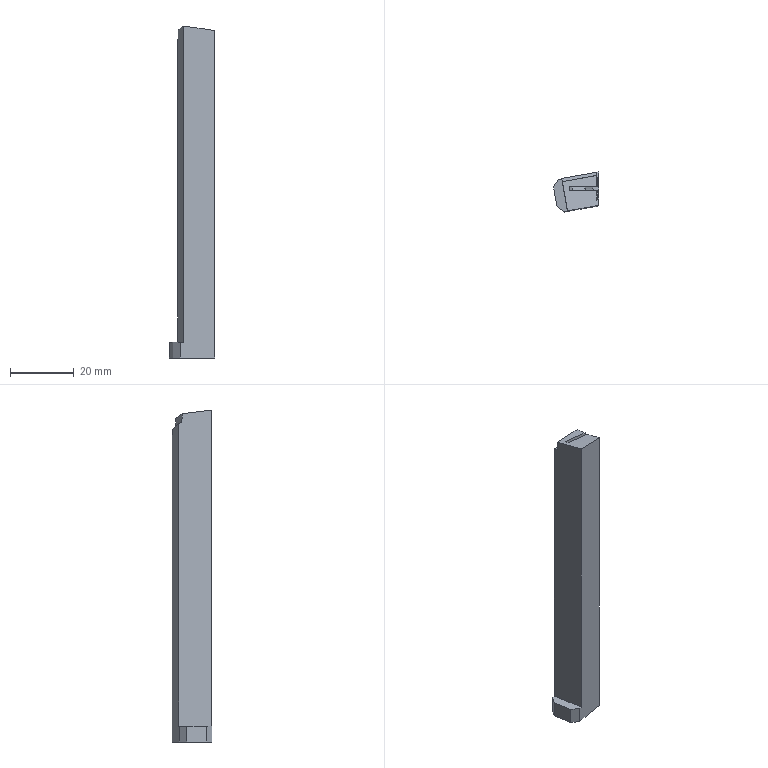Part | STEP file | P011002M004-000 | 1 solid | 27 faces | box 14.13 x 12.392 x 104.223 mm | volume 11432 mm3 | spline 24 | plane 3